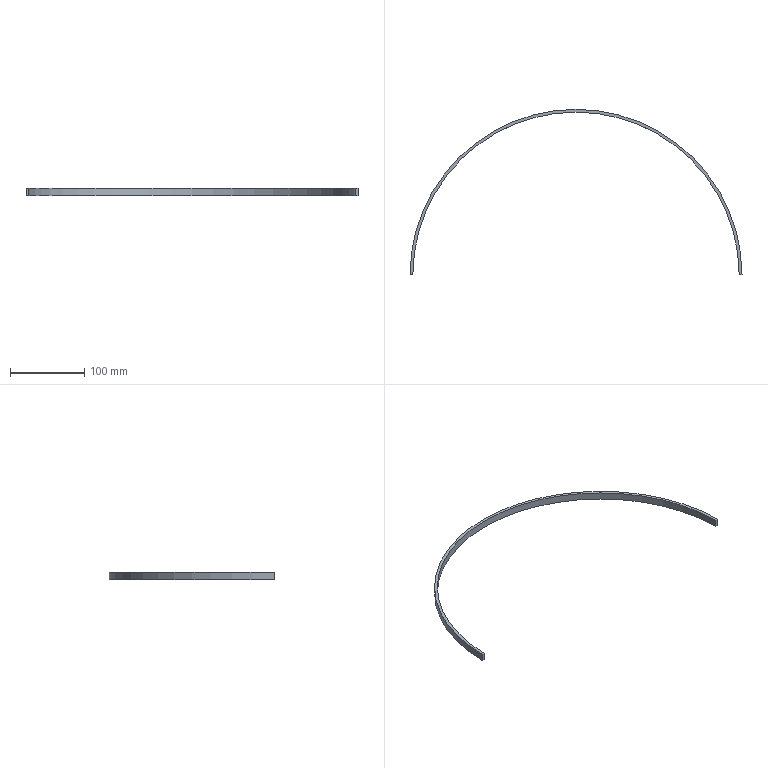Part | SolidWorks | features Extrusion 1 | 1 solid | 6 faces | box 447.996 x 223 x 10 mm | volume 26438 mm3 | plane 4 | cylinder 2 | commonest cylinder face diameters 440.4 x1 448 x1
STEP:
#1=CARTESIAN_POINT('',(443.998,1.,5.));
#2=VERTEX_POINT('',#1);
#3=CARTESIAN_POINT('',(-3.998,1.,5.));
#4=VERTEX_POINT('',#3);
#5=CARTESIAN_POINT('',(220.,0.,5.));
#6=DIRECTION('',(0.,0.,1.));
#7=DIRECTION('',(1.,0.,0.));
#8=AXIS2_PLACEMENT_3D('',#5,#6,#7);
#9=CIRCLE('',#8,224.);
#10=EDGE_CURVE('',#2,#4,#9,.T.);
#11=ORIENTED_EDGE('',*,*,#10,.F.);
#12=CARTESIAN_POINT('',(443.998,1.,-5.));
#13=VERTEX_POINT('',#12);
#14=CARTESIAN_POINT('',(443.998,1.,-5.));
#15=DIRECTION('',(0.,0.,1.));
#16=VECTOR('',#15,1000.);
#17=LINE('',#14,#16);
#18=EDGE_CURVE('',#13,#2,#17,.T.);
#19=ORIENTED_EDGE('',*,*,#18,.F.);
#20=CARTESIAN_POINT('',(-3.998,1.,-5.));
#21=VERTEX_POINT('',#20);
#22=CARTESIAN_POINT('',(220.,0.,-5.));
#23=DIRECTION('',(0.,0.,1.));
#24=DIRECTION('',(1.,0.,0.));
#25=AXIS2_PLACEMENT_3D('',#22,#23,#24);
#26=CIRCLE('',#25,224.);
#27=EDGE_CURVE('',#13,#21,#26,.T.);
#28=ORIENTED_EDGE('',*,*,#27,.T.);
#29=CARTESIAN_POINT('',(-3.998,1.,-5.));
#30=DIRECTION('',(0.,0.,1.));
#31=VECTOR('',#30,1000.);
#32=LINE('',#29,#31);
#33=EDGE_CURVE('',#21,#4,#32,.T.);
#34=ORIENTED_EDGE('',*,*,#33,.T.);
#35=EDGE_LOOP('',(#11,#19,#28,#34));
#36=FACE_OUTER_BOUND('',#35,.T.);
#37=CARTESIAN_POINT('',(220.,0.,-5.));
#38=DIRECTION('',(0.,0.,1.));
#39=DIRECTION('',(1.,0.,0.));
#40=AXIS2_PLACEMENT_3D('',#37,#38,#39);
#41=CYLINDRICAL_SURFACE('',#40,224.);
#42=ADVANCED_FACE('',(#36),#41,.T.);
#43=CARTESIAN_POINT('',(440.198,1.,5.));
#44=VERTEX_POINT('',#43);
#45=CARTESIAN_POINT('',(440.198,1.,5.));
#46=DIRECTION('',(1.,0.,0.));
#47=VECTOR('',#46,1000.);
#48=LINE('',#45,#47);
#49=EDGE_CURVE('',#44,#2,#48,.T.);
#50=ORIENTED_EDGE('',*,*,#49,.F.);
#51=CARTESIAN_POINT('',(440.198,1.,-5.));
#52=VERTEX_POINT('',#51);
#53=CARTESIAN_POINT('',(440.198,1.,-5.));
#54=DIRECTION('',(0.,0.,1.));
#55=VECTOR('',#54,1000.);
#56=LINE('',#53,#55);
#57=EDGE_CURVE('',#52,#44,#56,.T.);
#58=ORIENTED_EDGE('',*,*,#57,.F.);
#59=CARTESIAN_POINT('',(440.198,1.,-5.));
#60=DIRECTION('',(1.,0.,0.));
#61=VECTOR('',#60,1000.);
#62=LINE('',#59,#61);
#63=EDGE_CURVE('',#52,#13,#62,.T.);
#64=ORIENTED_EDGE('',*,*,#63,.T.);
#65=ORIENTED_EDGE('',*,*,#18,.T.);
#66=EDGE_LOOP('',(#50,#58,#64,#65));
#67=FACE_OUTER_BOUND('',#66,.T.);
#68=CARTESIAN_POINT('',(440.198,1.,-5.));
#69=DIRECTION('',(0.,-1.,0.));
#70=DIRECTION('',(1.,0.,0.));
#71=AXIS2_PLACEMENT_3D('',#68,#69,#70);
#72=PLANE('',#71);
#73=ADVANCED_FACE('',(#67),#72,.T.);
#74=CARTESIAN_POINT('',(-0.1977,1.,5.));
#75=VERTEX_POINT('',#74);
#76=CARTESIAN_POINT('',(220.,0.,5.));
#77=DIRECTION('',(0.,0.,-1.));
#78=DIRECTION('',(-1.,0.,0.));
#79=AXIS2_PLACEMENT_3D('',#76,#77,#78);
#80=CIRCLE('',#79,220.2);
#81=EDGE_CURVE('',#75,#44,#80,.T.);
#82=ORIENTED_EDGE('',*,*,#81,.F.);
#83=CARTESIAN_POINT('',(-0.1977,1.,-5.));
#84=VERTEX_POINT('',#83);
#85=CARTESIAN_POINT('',(-0.1977,1.,-5.));
#86=DIRECTION('',(0.,0.,1.));
#87=VECTOR('',#86,1000.);
#88=LINE('',#85,#87);
#89=EDGE_CURVE('',#84,#75,#88,.T.);
#90=ORIENTED_EDGE('',*,*,#89,.F.);
#91=CARTESIAN_POINT('',(220.,0.,-5.));
#92=DIRECTION('',(0.,0.,-1.));
#93=DIRECTION('',(-1.,0.,0.));
#94=AXIS2_PLACEMENT_3D('',#91,#92,#93);
#95=CIRCLE('',#94,220.2);
#96=EDGE_CURVE('',#84,#52,#95,.T.);
#97=ORIENTED_EDGE('',*,*,#96,.T.);
#98=ORIENTED_EDGE('',*,*,#57,.T.);
#99=EDGE_LOOP('',(#82,#90,#97,#98));
#100=FACE_OUTER_BOUND('',#99,.T.);
#101=CARTESIAN_POINT('',(220.,0.,-5.));
#102=DIRECTION('',(0.,0.,1.));
#103=DIRECTION('',(1.,0.,0.));
#104=AXIS2_PLACEMENT_3D('',#101,#102,#103);
#105=CYLINDRICAL_SURFACE('',#104,220.2);
#106=ADVANCED_FACE('',(#100),#105,.F.);
#107=CARTESIAN_POINT('',(-3.998,1.,5.));
#108=DIRECTION('',(1.,0.,0.));
#109=VECTOR('',#108,1000.);
#110=LINE('',#107,#109);
#111=EDGE_CURVE('',#4,#75,#110,.T.);
#112=ORIENTED_EDGE('',*,*,#111,.F.);
#113=ORIENTED_EDGE('',*,*,#33,.F.);
#114=CARTESIAN_POINT('',(-3.998,1.,-5.));
#115=DIRECTION('',(1.,0.,0.));
#116=VECTOR('',#115,1000.);
#117=LINE('',#114,#116);
#118=EDGE_CURVE('',#21,#84,#117,.T.);
#119=ORIENTED_EDGE('',*,*,#118,.T.);
#120=ORIENTED_EDGE('',*,*,#89,.T.);
#121=EDGE_LOOP('',(#112,#113,#119,#120));
#122=FACE_OUTER_BOUND('',#121,.T.);
#123=CARTESIAN_POINT('',(-3.998,1.,-5.));
#124=DIRECTION('',(0.,-1.,0.));
#125=DIRECTION('',(1.,0.,0.));
#126=AXIS2_PLACEMENT_3D('',#123,#124,#125);
#127=PLANE('',#126);
#128=ADVANCED_FACE('',(#122),#127,.T.);
#129=ORIENTED_EDGE('',*,*,#27,.F.);
#130=ORIENTED_EDGE('',*,*,#63,.F.);
#131=ORIENTED_EDGE('',*,*,#96,.F.);
#132=ORIENTED_EDGE('',*,*,#118,.F.);
#133=EDGE_LOOP('',(#129,#130,#131,#132));
#134=FACE_OUTER_BOUND('',#133,.T.);
#135=CARTESIAN_POINT('',(220.,0.,-5.));
#136=DIRECTION('',(0.,0.,1.));
#137=DIRECTION('',(1.,0.,0.));
#138=AXIS2_PLACEMENT_3D('',#135,#136,#137);
#139=PLANE('',#138);
#140=ADVANCED_FACE('',(#134),#139,.F.);
#141=ORIENTED_EDGE('',*,*,#10,.T.);
#142=ORIENTED_EDGE('',*,*,#111,.T.);
#143=ORIENTED_EDGE('',*,*,#81,.T.);
#144=ORIENTED_EDGE('',*,*,#49,.T.);
#145=EDGE_LOOP('',(#141,#142,#143,#144));
#146=FACE_OUTER_BOUND('',#145,.T.);
#147=CARTESIAN_POINT('',(220.,0.,5.));
#148=DIRECTION('',(0.,0.,1.));
#149=DIRECTION('',(1.,0.,0.));
#150=AXIS2_PLACEMENT_3D('',#147,#148,#149);
#151=PLANE('',#150);
#152=ADVANCED_FACE('',(#146),#151,.T.);
#153=CLOSED_SHELL('',(#42,#73,#106,#128,#140,#152));
#154=MANIFOLD_SOLID_BREP('',#153);
#155=CARTESIAN_POINT('',(0.,0.,0.));
#156=DIRECTION('',(0.,0.,1.));
#157=DIRECTION('',(1.,0.,0.));
#158=AXIS2_PLACEMENT_3D('',#155,#156,#157);
#159=(LENGTH_UNIT()NAMED_UNIT(*)SI_UNIT(.MILLI.,.METRE.));
#160=UNCERTAINTY_MEASURE_WITH_UNIT(LENGTH_MEASURE(0.00001),#159,'','');
#161=(NAMED_UNIT(*)PLANE_ANGLE_UNIT()SI_UNIT($,.RADIAN.));
#162=(NAMED_UNIT(*)SI_UNIT($,.STERADIAN.)SOLID_ANGLE_UNIT());
#163=(GEOMETRIC_REPRESENTATION_CONTEXT(3)GLOBAL_UNCERTAINTY_ASSIGNED_CONTEXT((#160))GLOBAL_UNIT_ASSIGNED_CONTEXT((#159,#161,#162))REPRESENTATION_CONTEXT('',''));
#164=ADVANCED_BREP_SHAPE_REPRESENTATION('',(#154,#158),#163);